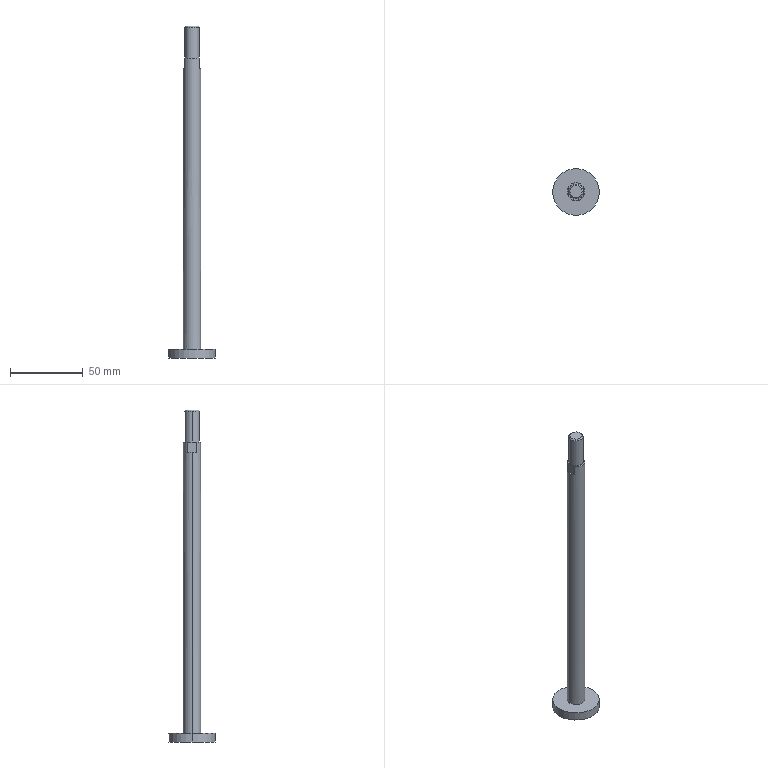Part | STEP file | 1 solid | 17 faces | box 32 x 32 x 228.2 mm | volume 29124 mm3 | plane 9 | cylinder 6 | cone 2 | commonest cylinder face diameters 10 x2 12 x2 32 x2
STEP:
#1=CARTESIAN_POINT('',(0.,0.,0.));
#2=DIRECTION('',(0.,0.,1.));
#3=DIRECTION('',(1.,0.,0.));
#4=AXIS2_PLACEMENT_3D('',#1,#2,#3);
#5=CARTESIAN_POINT('',(5.,0.,26.));
#6=VERTEX_POINT('',#5);
#7=CARTESIAN_POINT('',(-5.,0.,26.));
#8=VERTEX_POINT('',#7);
#9=CARTESIAN_POINT('',(0.,0.,26.));
#10=DIRECTION('',(0.,0.,1.));
#11=DIRECTION('',(1.,0.,0.));
#12=AXIS2_PLACEMENT_3D('',#9,#10,#11);
#13=CIRCLE('',#12,5.);
#14=CARTESIAN_POINT('',(0.,0.,26.));
#15=DIRECTION('',(0.,0.,1.));
#16=DIRECTION('',(1.,0.,0.));
#17=AXIS2_PLACEMENT_3D('',#14,#15,#16);
#18=CYLINDRICAL_SURFACE('',#17,5.);
#19=CARTESIAN_POINT('',(0.,0.));
#20=DIRECTION('',(1.,0.));
#21=VECTOR('',#20,1.);
#22=LINE('',#19,#21);
#23=(GEOMETRIC_REPRESENTATION_CONTEXT(2)PARAMETRIC_REPRESENTATION_CONTEXT()REPRESENTATION_CONTEXT('',''));
#24=DEFINITIONAL_REPRESENTATION('',(#22),#23);
#25=PCURVE('',#18,#24);
#26=CARTESIAN_POINT('',(0.,0.,26.));
#27=DIRECTION('',(0.,0.,-1.));
#28=DIRECTION('',(-1.,0.,0.));
#29=AXIS2_PLACEMENT_3D('',#26,#27,#28);
#30=PLANE('',#29);
#31=CARTESIAN_POINT('',(-5.,0.));
#32=CARTESIAN_POINT('',(-5.,8.66));
#33=CARTESIAN_POINT('',(2.5,4.33));
#34=CARTESIAN_POINT('',(10.,0.));
#35=CARTESIAN_POINT('',(2.5,-4.33));
#36=CARTESIAN_POINT('',(-5.,-8.66));
#37=CARTESIAN_POINT('',(-5.,0.));
#38=(BOUNDED_CURVE()B_SPLINE_CURVE(2,(#31,#32,#33,#34,#35,#36,#37),.UNSPECIFIED.,.T.,.F.)B_SPLINE_CURVE_WITH_KNOTS((1,2,2,2,2,1),(-2.094,0.,2.094,4.189,6.283,8.378),.UNSPECIFIED.)CURVE()GEOMETRIC_REPRESENTATION_ITEM()RATIONAL_B_SPLINE_CURVE((1.,0.5,1.,0.5,1.,0.5,1.))REPRESENTATION_ITEM(''));
#39=(GEOMETRIC_REPRESENTATION_CONTEXT(2)PARAMETRIC_REPRESENTATION_CONTEXT()REPRESENTATION_CONTEXT('',''));
#40=DEFINITIONAL_REPRESENTATION('',(#38),#39);
#41=PCURVE('',#30,#40);
#42=SURFACE_CURVE('',#13,(#25,#41),.PCURVE_S1.);
#43=EDGE_CURVE('',#6,#8,#42,.T.);
#44=ORIENTED_EDGE('',*,*,#43,.T.);
#45=CARTESIAN_POINT('',(-5.,0.,47.233));
#46=VERTEX_POINT('',#45);
#47=CARTESIAN_POINT('',(-5.,0.,26.));
#48=DIRECTION('',(0.,0.,1.));
#49=VECTOR('',#48,1.);
#50=LINE('',#47,#49);
#51=CARTESIAN_POINT('',(3.142,0.));
#52=DIRECTION('',(0.,1.));
#53=VECTOR('',#52,1.);
#54=LINE('',#51,#53);
#55=(GEOMETRIC_REPRESENTATION_CONTEXT(2)PARAMETRIC_REPRESENTATION_CONTEXT()REPRESENTATION_CONTEXT('',''));
#56=DEFINITIONAL_REPRESENTATION('',(#54),#55);
#57=PCURVE('',#18,#56);
#58=CARTESIAN_POINT('',(0.,0.,26.));
#59=DIRECTION('',(0.,0.,1.));
#60=DIRECTION('',(1.,0.,0.));
#61=AXIS2_PLACEMENT_3D('',#58,#59,#60);
#62=CYLINDRICAL_SURFACE('',#61,5.);
#63=CARTESIAN_POINT('',(3.142,0.));
#64=DIRECTION('',(0.,1.));
#65=VECTOR('',#64,1.);
#66=LINE('',#63,#65);
#67=(GEOMETRIC_REPRESENTATION_CONTEXT(2)PARAMETRIC_REPRESENTATION_CONTEXT()REPRESENTATION_CONTEXT('',''));
#68=DEFINITIONAL_REPRESENTATION('',(#66),#67);
#69=PCURVE('',#62,#68);
#70=SURFACE_CURVE('',#50,(#57,#69),.PCURVE_S1.);
#71=EDGE_CURVE('',#8,#46,#70,.T.);
#72=ORIENTED_EDGE('',*,*,#71,.T.);
#73=CARTESIAN_POINT('',(5.,0.,47.233));
#74=VERTEX_POINT('',#73);
#75=CARTESIAN_POINT('',(0.,0.,47.233));
#76=DIRECTION('',(0.,0.,1.));
#77=DIRECTION('',(1.,0.,0.));
#78=AXIS2_PLACEMENT_3D('',#75,#76,#77);
#79=CIRCLE('',#78,5.);
#80=CARTESIAN_POINT('',(0.,21.233));
#81=DIRECTION('',(1.,0.));
#82=VECTOR('',#81,1.);
#83=LINE('',#80,#82);
#84=(GEOMETRIC_REPRESENTATION_CONTEXT(2)PARAMETRIC_REPRESENTATION_CONTEXT()REPRESENTATION_CONTEXT('',''));
#85=DEFINITIONAL_REPRESENTATION('',(#83),#84);
#86=PCURVE('',#18,#85);
#87=CARTESIAN_POINT('',(0.,0.,47.233));
#88=DIRECTION('',(0.,0.,-1.));
#89=DIRECTION('',(-1.,0.,0.));
#90=AXIS2_PLACEMENT_3D('',#87,#88,#89);
#91=CONICAL_SURFACE('',#90,5.,0.7854);
#92=CARTESIAN_POINT('',(3.142,0.));
#93=DIRECTION('',(-1.,0.));
#94=VECTOR('',#93,1.);
#95=LINE('',#92,#94);
#96=(GEOMETRIC_REPRESENTATION_CONTEXT(2)PARAMETRIC_REPRESENTATION_CONTEXT()REPRESENTATION_CONTEXT('',''));
#97=DEFINITIONAL_REPRESENTATION('',(#95),#96);
#98=PCURVE('',#91,#97);
#99=SURFACE_CURVE('',#79,(#86,#98),.PCURVE_S1.);
#100=EDGE_CURVE('',#74,#46,#99,.T.);
#101=ORIENTED_EDGE('',*,*,#100,.F.);
#102=CARTESIAN_POINT('',(5.,0.,26.));
#103=DIRECTION('',(0.,0.,1.));
#104=VECTOR('',#103,1.);
#105=LINE('',#102,#104);
#106=CARTESIAN_POINT('',(0.,0.));
#107=DIRECTION('',(0.,1.));
#108=VECTOR('',#107,1.);
#109=LINE('',#106,#108);
#110=(GEOMETRIC_REPRESENTATION_CONTEXT(2)PARAMETRIC_REPRESENTATION_CONTEXT()REPRESENTATION_CONTEXT('',''));
#111=DEFINITIONAL_REPRESENTATION('',(#109),#110);
#112=PCURVE('',#18,#111);
#113=CARTESIAN_POINT('',(6.283,0.));
#114=DIRECTION('',(0.,1.));
#115=VECTOR('',#114,1.);
#116=LINE('',#113,#115);
#117=(GEOMETRIC_REPRESENTATION_CONTEXT(2)PARAMETRIC_REPRESENTATION_CONTEXT()REPRESENTATION_CONTEXT('',''));
#118=DEFINITIONAL_REPRESENTATION('',(#116),#117);
#119=PCURVE('',#62,#118);
#120=SURFACE_CURVE('',#105,(#112,#119),.PCURVE_S1.);
#121=EDGE_CURVE('',#6,#74,#120,.T.);
#122=ORIENTED_EDGE('',*,*,#121,.F.);
#123=EDGE_LOOP('',(#44,#72,#101,#122));
#124=FACE_BOUND('',#123,.T.);
#125=ADVANCED_FACE('',(#124),#18,.T.);
#126=CARTESIAN_POINT('',(4.233,0.,48.));
#127=VERTEX_POINT('',#126);
#128=CARTESIAN_POINT('',(-4.233,0.,48.));
#129=VERTEX_POINT('',#128);
#130=CARTESIAN_POINT('',(0.,0.,48.));
#131=DIRECTION('',(0.,0.,1.));
#132=DIRECTION('',(1.,0.,0.));
#133=AXIS2_PLACEMENT_3D('',#130,#131,#132);
#134=CIRCLE('',#133,4.233);
#135=CARTESIAN_POINT('',(3.142,-0.767));
#136=DIRECTION('',(-1.,0.));
#137=VECTOR('',#136,1.);
#138=LINE('',#135,#137);
#139=(GEOMETRIC_REPRESENTATION_CONTEXT(2)PARAMETRIC_REPRESENTATION_CONTEXT()REPRESENTATION_CONTEXT('',''));
#140=DEFINITIONAL_REPRESENTATION('',(#138),#139);
#141=PCURVE('',#91,#140);
#142=CARTESIAN_POINT('',(0.,0.,48.));
#143=DIRECTION('',(0.,0.,-1.));
#144=DIRECTION('',(-1.,0.,0.));
#145=AXIS2_PLACEMENT_3D('',#142,#143,#144);
#146=PLANE('',#145);
#147=CARTESIAN_POINT('',(-4.233,0.));
#148=CARTESIAN_POINT('',(-4.233,7.332));
#149=CARTESIAN_POINT('',(2.116,3.666));
#150=CARTESIAN_POINT('',(8.466,0.));
#151=CARTESIAN_POINT('',(2.116,-3.666));
#152=CARTESIAN_POINT('',(-4.233,-7.332));
#153=CARTESIAN_POINT('',(-4.233,0.));
#154=(BOUNDED_CURVE()B_SPLINE_CURVE(2,(#147,#148,#149,#150,#151,#152,#153),.UNSPECIFIED.,.T.,.F.)B_SPLINE_CURVE_WITH_KNOTS((1,2,2,2,2,1),(-2.094,0.,2.094,4.189,6.283,8.378),.UNSPECIFIED.)CURVE()GEOMETRIC_REPRESENTATION_ITEM()RATIONAL_B_SPLINE_CURVE((1.,0.5,1.,0.5,1.,0.5,1.))REPRESENTATION_ITEM(''));
#155=(GEOMETRIC_REPRESENTATION_CONTEXT(2)PARAMETRIC_REPRESENTATION_CONTEXT()REPRESENTATION_CONTEXT('',''));
#156=DEFINITIONAL_REPRESENTATION('',(#154),#155);
#157=PCURVE('',#146,#156);
#158=SURFACE_CURVE('',#134,(#141,#157),.PCURVE_S1.);
#159=EDGE_CURVE('',#127,#129,#158,.T.);
#160=ORIENTED_EDGE('',*,*,#159,.F.);
#161=CARTESIAN_POINT('',(5.,0.,47.233));
#162=DIRECTION('',(0.7071,0.,-0.7071));
#163=VECTOR('',#162,1.);
#164=LINE('',#161,#163);
#165=CARTESIAN_POINT('',(3.142,0.));
#166=DIRECTION('',(0.,1.));
#167=VECTOR('',#166,1.);
#168=LINE('',#165,#167);
#169=(GEOMETRIC_REPRESENTATION_CONTEXT(2)PARAMETRIC_REPRESENTATION_CONTEXT()REPRESENTATION_CONTEXT('',''));
#170=DEFINITIONAL_REPRESENTATION('',(#168),#169);
#171=PCURVE('',#91,#170);
#172=CARTESIAN_POINT('',(0.,0.,47.233));
#173=DIRECTION('',(0.,0.,-1.));
#174=DIRECTION('',(-1.,0.,0.));
#175=AXIS2_PLACEMENT_3D('',#172,#173,#174);
#176=CONICAL_SURFACE('',#175,5.,0.7854);
#177=CARTESIAN_POINT('',(3.142,0.));
#178=DIRECTION('',(0.,1.));
#179=VECTOR('',#178,1.);
#180=LINE('',#177,#179);
#181=(GEOMETRIC_REPRESENTATION_CONTEXT(2)PARAMETRIC_REPRESENTATION_CONTEXT()REPRESENTATION_CONTEXT('',''));
#182=DEFINITIONAL_REPRESENTATION('',(#180),#181);
#183=PCURVE('',#176,#182);
#184=SURFACE_CURVE('',#164,(#171,#183),.PCURVE_S1.);
#185=EDGE_CURVE('',#127,#74,#184,.T.);
#186=ORIENTED_EDGE('',*,*,#185,.T.);
#187=ORIENTED_EDGE('',*,*,#100,.T.);
#188=CARTESIAN_POINT('',(-5.,0.,47.233));
#189=DIRECTION('',(-0.7071,0.,-0.7071));
#190=VECTOR('',#189,1.);
#191=LINE('',#188,#190);
#192=CARTESIAN_POINT('',(0.,0.));
#193=DIRECTION('',(0.,1.));
#194=VECTOR('',#193,1.);
#195=LINE('',#192,#194);
#196=(GEOMETRIC_REPRESENTATION_CONTEXT(2)PARAMETRIC_REPRESENTATION_CONTEXT()REPRESENTATION_CONTEXT('',''));
#197=DEFINITIONAL_REPRESENTATION('',(#195),#196);
#198=PCURVE('',#91,#197);
#199=CARTESIAN_POINT('',(6.283,0.));
#200=DIRECTION('',(0.,1.));
#201=VECTOR('',#200,1.);
#202=LINE('',#199,#201);
#203=(GEOMETRIC_REPRESENTATION_CONTEXT(2)PARAMETRIC_REPRESENTATION_CONTEXT()REPRESENTATION_CONTEXT('',''));
#204=DEFINITIONAL_REPRESENTATION('',(#202),#203);
#205=PCURVE('',#176,#204);
#206=SURFACE_CURVE('',#191,(#198,#205),.PCURVE_S1.);
#207=EDGE_CURVE('',#129,#46,#206,.T.);
#208=ORIENTED_EDGE('',*,*,#207,.F.);
#209=EDGE_LOOP('',(#160,#186,#187,#208));
#210=FACE_BOUND('',#209,.T.);
#211=ADVANCED_FACE('',(#210),#91,.T.);
#212=CARTESIAN_POINT('',(16.,0.,-180.2));
#213=VERTEX_POINT('',#212);
#214=CARTESIAN_POINT('',(-16.,0.,-180.2));
#215=VERTEX_POINT('',#214);
#216=CARTESIAN_POINT('',(0.,0.,-180.2));
#217=DIRECTION('',(0.,0.,1.));
#218=DIRECTION('',(1.,0.,0.));
#219=AXIS2_PLACEMENT_3D('',#216,#217,#218);
#220=CIRCLE('',#219,16.);
#221=CARTESIAN_POINT('',(0.,0.,-180.2));
#222=DIRECTION('',(0.,0.,1.));
#223=DIRECTION('',(1.,0.,0.));
#224=AXIS2_PLACEMENT_3D('',#221,#222,#223);
#225=CYLINDRICAL_SURFACE('',#224,16.);
#226=CARTESIAN_POINT('',(0.,0.));
#227=DIRECTION('',(1.,0.));
#228=VECTOR('',#227,1.);
#229=LINE('',#226,#228);
#230=(GEOMETRIC_REPRESENTATION_CONTEXT(2)PARAMETRIC_REPRESENTATION_CONTEXT()REPRESENTATION_CONTEXT('',''));
#231=DEFINITIONAL_REPRESENTATION('',(#229),#230);
#232=PCURVE('',#225,#231);
#233=CARTESIAN_POINT('',(0.,16.,-180.2));
#234=DIRECTION('',(0.,0.,1.));
#235=DIRECTION('',(1.,0.,0.));
#236=AXIS2_PLACEMENT_3D('',#233,#234,#235);
#237=PLANE('',#236);
#238=CARTESIAN_POINT('',(0.,-16.));
#239=DIRECTION('',(1.,0.));
#240=AXIS2_PLACEMENT_2D('',#238,#239);
#241=CIRCLE('',#240,16.);
#242=(GEOMETRIC_REPRESENTATION_CONTEXT(2)PARAMETRIC_REPRESENTATION_CONTEXT()REPRESENTATION_CONTEXT('',''));
#243=DEFINITIONAL_REPRESENTATION('',(#241),#242);
#244=PCURVE('',#237,#243);
#245=SURFACE_CURVE('',#220,(#232,#244),.PCURVE_S1.);
#246=EDGE_CURVE('',#213,#215,#245,.T.);
#247=ORIENTED_EDGE('',*,*,#246,.T.);
#248=CARTESIAN_POINT('',(-16.,0.,-174.2));
#249=VERTEX_POINT('',#248);
#250=CARTESIAN_POINT('',(-16.,0.,-180.2));
#251=DIRECTION('',(0.,0.,1.));
#252=VECTOR('',#251,1.);
#253=LINE('',#250,#252);
#254=CARTESIAN_POINT('',(3.142,0.));
#255=DIRECTION('',(0.,1.));
#256=VECTOR('',#255,1.);
#257=LINE('',#254,#256);
#258=(GEOMETRIC_REPRESENTATION_CONTEXT(2)PARAMETRIC_REPRESENTATION_CONTEXT()REPRESENTATION_CONTEXT('',''));
#259=DEFINITIONAL_REPRESENTATION('',(#257),#258);
#260=PCURVE('',#225,#259);
#261=CARTESIAN_POINT('',(0.,0.,-180.2));
#262=DIRECTION('',(0.,0.,1.));
#263=DIRECTION('',(1.,0.,0.));
#264=AXIS2_PLACEMENT_3D('',#261,#262,#263);
#265=CYLINDRICAL_SURFACE('',#264,16.);
#266=CARTESIAN_POINT('',(3.142,0.));
#267=DIRECTION('',(0.,1.));
#268=VECTOR('',#267,1.);
#269=LINE('',#266,#268);
#270=(GEOMETRIC_REPRESENTATION_CONTEXT(2)PARAMETRIC_REPRESENTATION_CONTEXT()REPRESENTATION_CONTEXT('',''));
#271=DEFINITIONAL_REPRESENTATION('',(#269),#270);
#272=PCURVE('',#265,#271);
#273=SURFACE_CURVE('',#253,(#260,#272),.PCURVE_S1.);
#274=EDGE_CURVE('',#215,#249,#273,.T.);
#275=ORIENTED_EDGE('',*,*,#274,.T.);
#276=CARTESIAN_POINT('',(16.,0.,-174.2));
#277=VERTEX_POINT('',#276);
#278=CARTESIAN_POINT('',(0.,0.,-174.2));
#279=DIRECTION('',(0.,0.,1.));
#280=DIRECTION('',(1.,0.,0.));
#281=AXIS2_PLACEMENT_3D('',#278,#279,#280);
#282=CIRCLE('',#281,16.);
#283=CARTESIAN_POINT('',(0.,6.));
#284=DIRECTION('',(1.,0.));
#285=VECTOR('',#284,1.);
#286=LINE('',#283,#285);
#287=(GEOMETRIC_REPRESENTATION_CONTEXT(2)PARAMETRIC_REPRESENTATION_CONTEXT()REPRESENTATION_CONTEXT('',''));
#288=DEFINITIONAL_REPRESENTATION('',(#286),#287);
#289=PCURVE('',#225,#288);
#290=CARTESIAN_POINT('',(0.,6.,-174.2));
#291=DIRECTION('',(0.,0.,-1.));
#292=DIRECTION('',(-1.,0.,0.));
#293=AXIS2_PLACEMENT_3D('',#290,#291,#292);
#294=PLANE('',#293);
#295=CARTESIAN_POINT('',(-16.,-6.));
#296=CARTESIAN_POINT('',(-16.,21.713));
#297=CARTESIAN_POINT('',(8.,7.856));
#298=CARTESIAN_POINT('',(32.,-6.));
#299=CARTESIAN_POINT('',(8.,-19.856));
#300=CARTESIAN_POINT('',(-16.,-33.713));
#301=CARTESIAN_POINT('',(-16.,-6.));
#302=(BOUNDED_CURVE()B_SPLINE_CURVE(2,(#295,#296,#297,#298,#299,#300,#301),.UNSPECIFIED.,.T.,.F.)B_SPLINE_CURVE_WITH_KNOTS((1,2,2,2,2,1),(-2.094,0.,2.094,4.189,6.283,8.378),.UNSPECIFIED.)CURVE()GEOMETRIC_REPRESENTATION_ITEM()RATIONAL_B_SPLINE_CURVE((1.,0.5,1.,0.5,1.,0.5,1.))REPRESENTATION_ITEM(''));
#303=(GEOMETRIC_REPRESENTATION_CONTEXT(2)PARAMETRIC_REPRESENTATION_CONTEXT()REPRESENTATION_CONTEXT('',''));
#304=DEFINITIONAL_REPRESENTATION('',(#302),#303);
#305=PCURVE('',#294,#304);
#306=SURFACE_CURVE('',#282,(#289,#305),.PCURVE_S1.);
#307=EDGE_CURVE('',#277,#249,#306,.T.);
#308=ORIENTED_EDGE('',*,*,#307,.F.);
#309=CARTESIAN_POINT('',(16.,0.,-180.2));
#310=DIRECTION('',(0.,0.,1.));
#311=VECTOR('',#310,1.);
#312=LINE('',#309,#311);
#313=CARTESIAN_POINT('',(0.,0.));
#314=DIRECTION('',(0.,1.));
#315=VECTOR('',#314,1.);
#316=LINE('',#313,#315);
#317=(GEOMETRIC_REPRESENTATION_CONTEXT(2)PARAMETRIC_REPRESENTATION_CONTEXT()REPRESENTATION_CONTEXT('',''));
#318=DEFINITIONAL_REPRESENTATION('',(#316),#317);
#319=PCURVE('',#225,#318);
#320=CARTESIAN_POINT('',(6.283,0.));
#321=DIRECTION('',(0.,1.));
#322=VECTOR('',#321,1.);
#323=LINE('',#320,#322);
#324=(GEOMETRIC_REPRESENTATION_CONTEXT(2)PARAMETRIC_REPRESENTATION_CONTEXT()REPRESENTATION_CONTEXT('',''));
#325=DEFINITIONAL_REPRESENTATION('',(#323),#324);
#326=PCURVE('',#265,#325);
#327=SURFACE_CURVE('',#312,(#319,#326),.PCURVE_S1.);
#328=EDGE_CURVE('',#213,#277,#327,.T.);
#329=ORIENTED_EDGE('',*,*,#328,.F.);
#330=EDGE_LOOP('',(#247,#275,#308,#329));
#331=FACE_BOUND('',#330,.T.);
#332=ADVANCED_FACE('',(#331),#225,.T.);
#333=CARTESIAN_POINT('',(6.,0.,-174.2));
#334=VERTEX_POINT('',#333);
#335=CARTESIAN_POINT('',(-6.,0.,-174.2));
#336=VERTEX_POINT('',#335);
#337=CARTESIAN_POINT('',(0.,0.,-174.2));
#338=DIRECTION('',(0.,0.,1.));
#339=DIRECTION('',(1.,0.,0.));
#340=AXIS2_PLACEMENT_3D('',#337,#338,#339);
#341=CIRCLE('',#340,6.);
#342=CARTESIAN_POINT('',(0.,0.,-180.2));
#343=DIRECTION('',(0.,0.,1.));
#344=DIRECTION('',(1.,0.,0.));
#345=AXIS2_PLACEMENT_3D('',#342,#343,#344);
#346=CYLINDRICAL_SURFACE('',#345,6.);
#347=CARTESIAN_POINT('',(0.,6.));
#348=DIRECTION('',(1.,0.));
#349=VECTOR('',#348,1.);
#350=LINE('',#347,#349);
#351=(GEOMETRIC_REPRESENTATION_CONTEXT(2)PARAMETRIC_REPRESENTATION_CONTEXT()REPRESENTATION_CONTEXT('',''));
#352=DEFINITIONAL_REPRESENTATION('',(#350),#351);
#353=PCURVE('',#346,#352);
#354=CARTESIAN_POINT('',(-6.,-6.));
#355=CARTESIAN_POINT('',(-6.,4.392));
#356=CARTESIAN_POINT('',(3.,-0.8038));
#357=CARTESIAN_POINT('',(12.,-6.));
#358=CARTESIAN_POINT('',(3.,-11.196));
#359=CARTESIAN_POINT('',(-6.,-16.392));
#360=CARTESIAN_POINT('',(-6.,-6.));
#361=(BOUNDED_CURVE()B_SPLINE_CURVE(2,(#354,#355,#356,#357,#358,#359,#360),.UNSPECIFIED.,.T.,.F.)B_SPLINE_CURVE_WITH_KNOTS((1,2,2,2,2,1),(-2.094,0.,2.094,4.189,6.283,8.378),.UNSPECIFIED.)CURVE()GEOMETRIC_REPRESENTATION_ITEM()RATIONAL_B_SPLINE_CURVE((1.,0.5,1.,0.5,1.,0.5,1.))REPRESENTATION_ITEM(''));
#362=(GEOMETRIC_REPRESENTATION_CONTEXT(2)PARAMETRIC_REPRESENTATION_CONTEXT()REPRESENTATION_CONTEXT('',''));
#363=DEFINITIONAL_REPRESENTATION('',(#361),#362);
#364=PCURVE('',#294,#363);
#365=SURFACE_CURVE('',#341,(#353,#364),.PCURVE_S1.);
#366=EDGE_CURVE('',#334,#336,#365,.T.);
#367=ORIENTED_EDGE('',*,*,#366,.T.);
#368=CARTESIAN_POINT('',(-6.,0.,19.));
#369=VERTEX_POINT('',#368);
#370=CARTESIAN_POINT('',(-6.,0.,-180.2));
#371=DIRECTION('',(0.,0.,1.));
#372=VECTOR('',#371,1.);
#373=LINE('',#370,#372);
#374=CARTESIAN_POINT('',(3.142,0.));
#375=DIRECTION('',(0.,1.));
#376=VECTOR('',#375,1.);
#377=LINE('',#374,#376);
#378=(GEOMETRIC_REPRESENTATION_CONTEXT(2)PARAMETRIC_REPRESENTATION_CONTEXT()REPRESENTATION_CONTEXT('',''));
#379=DEFINITIONAL_REPRESENTATION('',(#377),#378);
#380=PCURVE('',#346,#379);
#381=CARTESIAN_POINT('',(0.,0.,-180.2));
#382=DIRECTION('',(0.,0.,1.));
#383=DIRECTION('',(1.,0.,0.));
#384=AXIS2_PLACEMENT_3D('',#381,#382,#383);
#385=CYLINDRICAL_SURFACE('',#384,6.);
#386=CARTESIAN_POINT('',(3.142,0.));
#387=DIRECTION('',(0.,1.));
#388=VECTOR('',#387,1.);
#389=LINE('',#386,#388);
#390=(GEOMETRIC_REPRESENTATION_CONTEXT(2)PARAMETRIC_REPRESENTATION_CONTEXT()REPRESENTATION_CONTEXT('',''));
#391=DEFINITIONAL_REPRESENTATION('',(#389),#390);
#392=PCURVE('',#385,#391);
#393=SURFACE_CURVE('',#373,(#380,#392),.PCURVE_S1.);
#394=EDGE_CURVE('',#336,#369,#393,.T.);
#395=ORIENTED_EDGE('',*,*,#394,.T.);
#396=CARTESIAN_POINT('',(-5.,3.317,19.));
#397=VERTEX_POINT('',#396);
#398=CARTESIAN_POINT('',(0.,0.,19.));
#399=DIRECTION('',(0.,0.,1.));
#400=DIRECTION('',(1.,0.,0.));
#401=AXIS2_PLACEMENT_3D('',#398,#399,#400);
#402=CIRCLE('',#401,6.);
#403=CARTESIAN_POINT('',(0.,199.2));
#404=DIRECTION('',(1.,0.));
#405=VECTOR('',#404,1.);
#406=LINE('',#403,#405);
#407=(GEOMETRIC_REPRESENTATION_CONTEXT(2)PARAMETRIC_REPRESENTATION_CONTEXT()REPRESENTATION_CONTEXT('',''));
#408=DEFINITIONAL_REPRESENTATION('',(#406),#407);
#409=PCURVE('',#346,#408);
#410=CARTESIAN_POINT('',(0.,0.,19.));
#411=DIRECTION('',(0.,0.,1.));
#412=DIRECTION('',(1.,0.,0.));
#413=AXIS2_PLACEMENT_3D('',#410,#411,#412);
#414=PLANE('',#413);
#415=CARTESIAN_POINT('',(0.,0.));
#416=DIRECTION('',(1.,0.));
#417=AXIS2_PLACEMENT_2D('',#415,#416);
#418=CIRCLE('',#417,6.);
#419=(GEOMETRIC_REPRESENTATION_CONTEXT(2)PARAMETRIC_REPRESENTATION_CONTEXT()REPRESENTATION_CONTEXT('',''));
#420=DEFINITIONAL_REPRESENTATION('',(#418),#419);
#421=PCURVE('',#414,#420);
#422=SURFACE_CURVE('',#402,(#409,#421),.PCURVE_S1.);
#423=EDGE_CURVE('',#397,#369,#422,.T.);
#424=ORIENTED_EDGE('',*,*,#423,.F.);
#425=CARTESIAN_POINT('',(-5.,3.317,26.));
#426=VERTEX_POINT('',#425);
#427=CARTESIAN_POINT('',(-5.,3.317,-180.2));
#428=DIRECTION('',(0.,0.,1.));
#429=VECTOR('',#428,1.);
#430=LINE('',#427,#429);
#431=CARTESIAN_POINT('',(2.556,0.));
#432=DIRECTION('',(0.,1.));
#433=VECTOR('',#432,1.);
#434=LINE('',#431,#433);
#435=(GEOMETRIC_REPRESENTATION_CONTEXT(2)PARAMETRIC_REPRESENTATION_CONTEXT()REPRESENTATION_CONTEXT('',''));
#436=DEFINITIONAL_REPRESENTATION('',(#434),#435);
#437=PCURVE('',#346,#436);
#438=CARTESIAN_POINT('',(-5.,-10.,19.));
#439=DIRECTION('',(1.,0.,0.));
#440=DIRECTION('',(0.,0.,-1.));
#441=AXIS2_PLACEMENT_3D('',#438,#439,#440);
#442=PLANE('',#441);
#443=CARTESIAN_POINT('',(199.2,13.317));
#444=DIRECTION('',(-1.,0.));
#445=VECTOR('',#444,1.);
#446=LINE('',#443,#445);
#447=(GEOMETRIC_REPRESENTATION_CONTEXT(2)PARAMETRIC_REPRESENTATION_CONTEXT()REPRESENTATION_CONTEXT('',''));
#448=DEFINITIONAL_REPRESENTATION('',(#446),#447);
#449=PCURVE('',#442,#448);
#450=SURFACE_CURVE('',#430,(#437,#449),.PCURVE_S1.);
#451=EDGE_CURVE('',#397,#426,#450,.T.);
#452=ORIENTED_EDGE('',*,*,#451,.T.);
#453=CARTESIAN_POINT('',(5.,3.317,26.));
#454=VERTEX_POINT('',#453);
#455=CARTESIAN_POINT('',(0.,0.,26.));
#456=DIRECTION('',(0.,0.,1.));
#457=DIRECTION('',(1.,0.,0.));
#458=AXIS2_PLACEMENT_3D('',#455,#456,#457);
#459=CIRCLE('',#458,6.);
#460=CARTESIAN_POINT('',(0.,206.2));
#461=DIRECTION('',(1.,0.));
#462=VECTOR('',#461,1.);
#463=LINE('',#460,#462);
#464=(GEOMETRIC_REPRESENTATION_CONTEXT(2)PARAMETRIC_REPRESENTATION_CONTEXT()REPRESENTATION_CONTEXT('',''));
#465=DEFINITIONAL_REPRESENTATION('',(#463),#464);
#466=PCURVE('',#346,#465);
#467=CARTESIAN_POINT('',(-6.,0.));
#468=CARTESIAN_POINT('',(-6.,10.392));
#469=CARTESIAN_POINT('',(3.,5.196));
#470=CARTESIAN_POINT('',(12.,0.));
#471=CARTESIAN_POINT('',(3.,-5.196));
#472=CARTESIAN_POINT('',(-6.,-10.392));
#473=CARTESIAN_POINT('',(-6.,0.));
#474=(BOUNDED_CURVE()B_SPLINE_CURVE(2,(#467,#468,#469,#470,#471,#472,#473),.UNSPECIFIED.,.T.,.F.)B_SPLINE_CURVE_WITH_KNOTS((1,2,2,2,2,1),(-2.094,0.,2.094,4.189,6.283,8.378),.UNSPECIFIED.)CURVE()GEOMETRIC_REPRESENTATION_ITEM()RATIONAL_B_SPLINE_CURVE((1.,0.5,1.,0.5,1.,0.5,1.))REPRESENTATION_ITEM(''));
#475=(GEOMETRIC_REPRESENTATION_CONTEXT(2)PARAMETRIC_REPRESENTATION_CONTEXT()REPRESENTATION_CONTEXT('',''));
#476=DEFINITIONAL_REPRESENTATION('',(#474),#475);
#477=PCURVE('',#30,#476);
#478=SURFACE_CURVE('',#459,(#466,#477),.PCURVE_S1.);
#479=EDGE_CURVE('',#454,#426,#478,.T.);
#480=ORIENTED_EDGE('',*,*,#479,.F.);
#481=CARTESIAN_POINT('',(5.,3.317,19.));
#482=VERTEX_POINT('',#481);
#483=CARTESIAN_POINT('',(5.,3.317,-180.2));
#484=DIRECTION('',(0.,0.,-1.));
#485=VECTOR('',#484,1.);
#486=LINE('',#483,#485);
#487=CARTESIAN_POINT('',(0.5857,0.));
#488=DIRECTION('',(0.,-1.));
#489=VECTOR('',#488,1.);
#490=LINE('',#487,#489);
#491=(GEOMETRIC_REPRESENTATION_CONTEXT(2)PARAMETRIC_REPRESENTATION_CONTEXT()REPRESENTATION_CONTEXT('',''));
#492=DEFINITIONAL_REPRESENTATION('',(#490),#491);
#493=PCURVE('',#346,#492);
#494=CARTESIAN_POINT('',(5.,10.,19.));
#495=DIRECTION('',(-1.,0.,0.));
#496=DIRECTION('',(0.,0.,1.));
#497=AXIS2_PLACEMENT_3D('',#494,#495,#496);
#498=PLANE('',#497);
#499=CARTESIAN_POINT('',(-199.2,-6.683));
#500=DIRECTION('',(-1.,0.));
#501=VECTOR('',#500,1.);
#502=LINE('',#499,#501);
#503=(GEOMETRIC_REPRESENTATION_CONTEXT(2)PARAMETRIC_REPRESENTATION_CONTEXT()REPRESENTATION_CONTEXT('',''));
#504=DEFINITIONAL_REPRESENTATION('',(#502),#503);
#505=PCURVE('',#498,#504);
#506=SURFACE_CURVE('',#486,(#493,#505),.PCURVE_S1.);
#507=EDGE_CURVE('',#454,#482,#506,.T.);
#508=ORIENTED_EDGE('',*,*,#507,.T.);
#509=CARTESIAN_POINT('',(6.,0.,19.));
#510=VERTEX_POINT('',#509);
#511=CARTESIAN_POINT('',(0.,0.,19.));
#512=DIRECTION('',(0.,0.,1.));
#513=DIRECTION('',(1.,0.,0.));
#514=AXIS2_PLACEMENT_3D('',#511,#512,#513);
#515=CIRCLE('',#514,6.);
#516=CARTESIAN_POINT('',(0.,199.2));
#517=DIRECTION('',(1.,0.));
#518=VECTOR('',#517,1.);
#519=LINE('',#516,#518);
#520=(GEOMETRIC_REPRESENTATION_CONTEXT(2)PARAMETRIC_REPRESENTATION_CONTEXT()REPRESENTATION_CONTEXT('',''));
#521=DEFINITIONAL_REPRESENTATION('',(#519),#520);
#522=PCURVE('',#346,#521);
#523=CARTESIAN_POINT('',(0.,0.,19.));
#524=DIRECTION('',(0.,0.,1.));
#525=DIRECTION('',(1.,0.,0.));
#526=AXIS2_PLACEMENT_3D('',#523,#524,#525);
#527=PLANE('',#526);
#528=CARTESIAN_POINT('',(0.,0.));
#529=DIRECTION('',(1.,0.));
#530=AXIS2_PLACEMENT_2D('',#528,#529);
#531=CIRCLE('',#530,6.);
#532=(GEOMETRIC_REPRESENTATION_CONTEXT(2)PARAMETRIC_REPRESENTATION_CONTEXT()REPRESENTATION_CONTEXT('',''));
#533=DEFINITIONAL_REPRESENTATION('',(#531),#532);
#534=PCURVE('',#527,#533);
#535=SURFACE_CURVE('',#515,(#522,#534),.PCURVE_S1.);
#536=EDGE_CURVE('',#510,#482,#535,.T.);
#537=ORIENTED_EDGE('',*,*,#536,.F.);
#538=CARTESIAN_POINT('',(6.,0.,-180.2));
#539=DIRECTION('',(0.,0.,1.));
#540=VECTOR('',#539,1.);
#541=LINE('',#538,#540);
#542=CARTESIAN_POINT('',(0.,0.));
#543=DIRECTION('',(0.,1.));
#544=VECTOR('',#543,1.);
#545=LINE('',#542,#544);
#546=(GEOMETRIC_REPRESENTATION_CONTEXT(2)PARAMETRIC_REPRESENTATION_CONTEXT()REPRESENTATION_CONTEXT('',''));
#547=DEFINITIONAL_REPRESENTATION('',(#545),#546);
#548=PCURVE('',#346,#547);
#549=CARTESIAN_POINT('',(6.283,0.));
#550=DIRECTION('',(0.,1.));
#551=VECTOR('',#550,1.);
#552=LINE('',#549,#551);
#553=(GEOMETRIC_REPRESENTATION_CONTEXT(2)PARAMETRIC_REPRESENTATION_CONTEXT()REPRESENTATION_CONTEXT('',''));
#554=DEFINITIONAL_REPRESENTATION('',(#552),#553);
#555=PCURVE('',#385,#554);
#556=SURFACE_CURVE('',#541,(#548,#555),.PCURVE_S1.);
#557=EDGE_CURVE('',#334,#510,#556,.T.);
#558=ORIENTED_EDGE('',*,*,#557,.F.);
#559=EDGE_LOOP('',(#367,#395,#424,#452,#480,#508,#537,#558));
#560=FACE_BOUND('',#559,.T.);
#561=ADVANCED_FACE('',(#560),#346,.T.);
#562=ORIENTED_EDGE('',*,*,#43,.F.);
#563=CARTESIAN_POINT('',(5.,10.,26.));
#564=DIRECTION('',(0.,-1.,0.));
#565=VECTOR('',#564,1.);
#566=LINE('',#563,#565);
#567=CARTESIAN_POINT('',(-5.,10.));
#568=DIRECTION('',(0.,-1.));
#569=VECTOR('',#568,1.);
#570=LINE('',#567,#569);
#571=(GEOMETRIC_REPRESENTATION_CONTEXT(2)PARAMETRIC_REPRESENTATION_CONTEXT()REPRESENTATION_CONTEXT('',''));
#572=DEFINITIONAL_REPRESENTATION('',(#570),#571);
#573=PCURVE('',#30,#572);
#574=CARTESIAN_POINT('',(7.,0.));
#575=DIRECTION('',(0.,-1.));
#576=VECTOR('',#575,1.);
#577=LINE('',#574,#576);
#578=(GEOMETRIC_REPRESENTATION_CONTEXT(2)PARAMETRIC_REPRESENTATION_CONTEXT()REPRESENTATION_CONTEXT('',''));
#579=DEFINITIONAL_REPRESENTATION('',(#577),#578);
#580=PCURVE('',#498,#579);
#581=SURFACE_CURVE('',#566,(#573,#580),.PCURVE_S1.);
#582=EDGE_CURVE('',#454,#6,#581,.T.);
#583=ORIENTED_EDGE('',*,*,#582,.F.);
#584=ORIENTED_EDGE('',*,*,#479,.T.);
#585=CARTESIAN_POINT('',(-5.,-10.,26.));
#586=DIRECTION('',(0.,1.,0.));
#587=VECTOR('',#586,1.);
#588=LINE('',#585,#587);
#589=CARTESIAN_POINT('',(5.,-10.));
#590=DIRECTION('',(0.,1.));
#591=VECTOR('',#590,1.);
#592=LINE('',#589,#591);
#593=(GEOMETRIC_REPRESENTATION_CONTEXT(2)PARAMETRIC_REPRESENTATION_CONTEXT()REPRESENTATION_CONTEXT('',''));
#594=DEFINITIONAL_REPRESENTATION('',(#592),#593);
#595=PCURVE('',#30,#594);
#596=CARTESIAN_POINT('',(-7.,0.));
#597=DIRECTION('',(0.,1.));
#598=VECTOR('',#597,1.);
#599=LINE('',#596,#598);
#600=(GEOMETRIC_REPRESENTATION_CONTEXT(2)PARAMETRIC_REPRESENTATION_CONTEXT()REPRESENTATION_CONTEXT('',''));
#601=DEFINITIONAL_REPRESENTATION('',(#599),#600);
#602=PCURVE('',#442,#601);
#603=SURFACE_CURVE('',#588,(#595,#602),.PCURVE_S1.);
#604=EDGE_CURVE('',#8,#426,#603,.T.);
#605=ORIENTED_EDGE('',*,*,#604,.F.);
#606=EDGE_LOOP('',(#562,#583,#584,#605));
#607=FACE_BOUND('',#606,.T.);
#608=ADVANCED_FACE('',(#607),#30,.F.);
#609=CARTESIAN_POINT('',(0.,0.,26.));
#610=DIRECTION('',(0.,0.,1.));
#611=DIRECTION('',(1.,0.,0.));
#612=AXIS2_PLACEMENT_3D('',#609,#610,#611);
#613=CIRCLE('',#612,5.);
#614=CARTESIAN_POINT('',(0.,0.,26.));
#615=DIRECTION('',(0.,0.,-1.));
#616=DIRECTION('',(-1.,0.,0.));
#617=AXIS2_PLACEMENT_3D('',#614,#615,#616);
#618=PLANE('',#617);
#619=CARTESIAN_POINT('',(-5.,0.));
#620=CARTESIAN_POINT('',(-5.,8.66));
#621=CARTESIAN_POINT('',(2.5,4.33));
#622=CARTESIAN_POINT('',(10.,0.));
#623=CARTESIAN_POINT('',(2.5,-4.33));
#624=CARTESIAN_POINT('',(-5.,-8.66));
#625=CARTESIAN_POINT('',(-5.,0.));
#626=(BOUNDED_CURVE()B_SPLINE_CURVE(2,(#619,#620,#621,#622,#623,#624,#625),.UNSPECIFIED.,.T.,.F.)B_SPLINE_CURVE_WITH_KNOTS((1,2,2,2,2,1),(-2.094,0.,2.094,4.189,6.283,8.378),.UNSPECIFIED.)CURVE()GEOMETRIC_REPRESENTATION_ITEM()RATIONAL_B_SPLINE_CURVE((1.,0.5,1.,0.5,1.,0.5,1.))REPRESENTATION_ITEM(''));
#627=(GEOMETRIC_REPRESENTATION_CONTEXT(2)PARAMETRIC_REPRESENTATION_CONTEXT()REPRESENTATION_CONTEXT('',''));
#628=DEFINITIONAL_REPRESENTATION('',(#626),#627);
#629=PCURVE('',#618,#628);
#630=CARTESIAN_POINT('',(0.,0.));
#631=DIRECTION('',(1.,0.));
#632=VECTOR('',#631,1.);
#633=LINE('',#630,#632);
#634=(GEOMETRIC_REPRESENTATION_CONTEXT(2)PARAMETRIC_REPRESENTATION_CONTEXT()REPRESENTATION_CONTEXT('',''));
#635=DEFINITIONAL_REPRESENTATION('',(#633),#634);
#636=PCURVE('',#62,#635);
#637=SURFACE_CURVE('',#613,(#629,#636),.PCURVE_S1.);
#638=EDGE_CURVE('',#8,#6,#637,.T.);
#639=ORIENTED_EDGE('',*,*,#638,.F.);
#640=CARTESIAN_POINT('',(-5.,-3.317,26.));
#641=VERTEX_POINT('',#640);
#642=CARTESIAN_POINT('',(-5.,-10.,26.));
#643=DIRECTION('',(0.,1.,0.));
#644=VECTOR('',#643,1.);
#645=LINE('',#642,#644);
#646=CARTESIAN_POINT('',(5.,-10.));
#647=DIRECTION('',(0.,1.));
#648=VECTOR('',#647,1.);
#649=LINE('',#646,#648);
#650=(GEOMETRIC_REPRESENTATION_CONTEXT(2)PARAMETRIC_REPRESENTATION_CONTEXT()REPRESENTATION_CONTEXT('',''));
#651=DEFINITIONAL_REPRESENTATION('',(#649),#650);
#652=PCURVE('',#618,#651);
#653=CARTESIAN_POINT('',(-7.,0.));
#654=DIRECTION('',(0.,1.));
#655=VECTOR('',#654,1.);
#656=LINE('',#653,#655);
#657=(GEOMETRIC_REPRESENTATION_CONTEXT(2)PARAMETRIC_REPRESENTATION_CONTEXT()REPRESENTATION_CONTEXT('',''));
#658=DEFINITIONAL_REPRESENTATION('',(#656),#657);
#659=PCURVE('',#442,#658);
#660=SURFACE_CURVE('',#645,(#652,#659),.PCURVE_S1.);
#661=EDGE_CURVE('',#641,#8,#660,.T.);
#662=ORIENTED_EDGE('',*,*,#661,.F.);
#663=CARTESIAN_POINT('',(5.,-3.317,26.));
#664=VERTEX_POINT('',#663);
#665=CARTESIAN_POINT('',(0.,0.,26.));
#666=DIRECTION('',(0.,0.,1.));
#667=DIRECTION('',(1.,0.,0.));
#668=AXIS2_PLACEMENT_3D('',#665,#666,#667);
#669=CIRCLE('',#668,6.);
#670=CARTESIAN_POINT('',(-6.,0.));
#671=CARTESIAN_POINT('',(-6.,10.392));
#672=CARTESIAN_POINT('',(3.,5.196));
#673=CARTESIAN_POINT('',(12.,0.));
#674=CARTESIAN_POINT('',(3.,-5.196));
#675=CARTESIAN_POINT('',(-6.,-10.392));
#676=CARTESIAN_POINT('',(-6.,0.));
#677=(BOUNDED_CURVE()B_SPLINE_CURVE(2,(#670,#671,#672,#673,#674,#675,#676),.UNSPECIFIED.,.T.,.F.)B_SPLINE_CURVE_WITH_KNOTS((1,2,2,2,2,1),(-2.094,0.,2.094,4.189,6.283,8.378),.UNSPECIFIED.)CURVE()GEOMETRIC_REPRESENTATION_ITEM()RATIONAL_B_SPLINE_CURVE((1.,0.5,1.,0.5,1.,0.5,1.))REPRESENTATION_ITEM(''));
#678=(GEOMETRIC_REPRESENTATION_CONTEXT(2)PARAMETRIC_REPRESENTATION_CONTEXT()REPRESENTATION_CONTEXT('',''));
#679=DEFINITIONAL_REPRESENTATION('',(#677),#678);
#680=PCURVE('',#618,#679);
#681=CARTESIAN_POINT('',(0.,206.2));
#682=DIRECTION('',(1.,0.));
#683=VECTOR('',#682,1.);
#684=LINE('',#681,#683);
#685=(GEOMETRIC_REPRESENTATION_CONTEXT(2)PARAMETRIC_REPRESENTATION_CONTEXT()REPRESENTATION_CONTEXT('',''));
#686=DEFINITIONAL_REPRESENTATION('',(#684),#685);
#687=PCURVE('',#385,#686);
#688=SURFACE_CURVE('',#669,(#680,#687),.PCURVE_S1.);
#689=EDGE_CURVE('',#641,#664,#688,.T.);
#690=ORIENTED_EDGE('',*,*,#689,.T.);
#691=CARTESIAN_POINT('',(5.,10.,26.));
#692=DIRECTION('',(0.,-1.,0.));
#693=VECTOR('',#692,1.);
#694=LINE('',#691,#693);
#695=CARTESIAN_POINT('',(-5.,10.));
#696=DIRECTION('',(0.,-1.));
#697=VECTOR('',#696,1.);
#698=LINE('',#695,#697);
#699=(GEOMETRIC_REPRESENTATION_CONTEXT(2)PARAMETRIC_REPRESENTATION_CONTEXT()REPRESENTATION_CONTEXT('',''));
#700=DEFINITIONAL_REPRESENTATION('',(#698),#699);
#701=PCURVE('',#618,#700);
#702=CARTESIAN_POINT('',(7.,0.));
#703=DIRECTION('',(0.,-1.));
#704=VECTOR('',#703,1.);
#705=LINE('',#702,#704);
#706=(GEOMETRIC_REPRESENTATION_CONTEXT(2)PARAMETRIC_REPRESENTATION_CONTEXT()REPRESENTATION_CONTEXT('',''));
#707=DEFINITIONAL_REPRESENTATION('',(#705),#706);
#708=PCURVE('',#498,#707);
#709=SURFACE_CURVE('',#694,(#701,#708),.PCURVE_S1.);
#710=EDGE_CURVE('',#6,#664,#709,.T.);
#711=ORIENTED_EDGE('',*,*,#710,.F.);
#712=EDGE_LOOP('',(#639,#662,#690,#711));
#713=FACE_BOUND('',#712,.T.);
#714=ADVANCED_FACE('',(#713),#618,.F.);
#715=ORIENTED_EDGE('',*,*,#394,.F.);
#716=CARTESIAN_POINT('',(0.,0.,-174.2));
#717=DIRECTION('',(0.,0.,1.));
#718=DIRECTION('',(1.,0.,0.));
#719=AXIS2_PLACEMENT_3D('',#716,#717,#718);
#720=CIRCLE('',#719,6.);
#721=CARTESIAN_POINT('',(0.,6.));
#722=DIRECTION('',(1.,0.));
#723=VECTOR('',#722,1.);
#724=LINE('',#721,#723);
#725=(GEOMETRIC_REPRESENTATION_CONTEXT(2)PARAMETRIC_REPRESENTATION_CONTEXT()REPRESENTATION_CONTEXT('',''));
#726=DEFINITIONAL_REPRESENTATION('',(#724),#725);
#727=PCURVE('',#385,#726);
#728=CARTESIAN_POINT('',(-6.,-6.));
#729=CARTESIAN_POINT('',(-6.,4.392));
#730=CARTESIAN_POINT('',(3.,-0.8038));
#731=CARTESIAN_POINT('',(12.,-6.));
#732=CARTESIAN_POINT('',(3.,-11.196));
#733=CARTESIAN_POINT('',(-6.,-16.392));
#734=CARTESIAN_POINT('',(-6.,-6.));
#735=(BOUNDED_CURVE()B_SPLINE_CURVE(2,(#728,#729,#730,#731,#732,#733,#734),.UNSPECIFIED.,.T.,.F.)B_SPLINE_CURVE_WITH_KNOTS((1,2,2,2,2,1),(-2.094,0.,2.094,4.189,6.283,8.378),.UNSPECIFIED.)CURVE()GEOMETRIC_REPRESENTATION_ITEM()RATIONAL_B_SPLINE_CURVE((1.,0.5,1.,0.5,1.,0.5,1.))REPRESENTATION_ITEM(''));
#736=(GEOMETRIC_REPRESENTATION_CONTEXT(2)PARAMETRIC_REPRESENTATION_CONTEXT()REPRESENTATION_CONTEXT('',''));
#737=DEFINITIONAL_REPRESENTATION('',(#735),#736);
#738=PCURVE('',#294,#737);
#739=SURFACE_CURVE('',#720,(#727,#738),.PCURVE_S1.);
#740=EDGE_CURVE('',#336,#334,#739,.T.);
#741=ORIENTED_EDGE('',*,*,#740,.T.);
#742=ORIENTED_EDGE('',*,*,#557,.T.);
#743=CARTESIAN_POINT('',(5.,-3.317,19.));
#744=VERTEX_POINT('',#743);
#745=CARTESIAN_POINT('',(0.,0.,19.));
#746=DIRECTION('',(0.,0.,1.));
#747=DIRECTION('',(1.,0.,0.));
#748=AXIS2_PLACEMENT_3D('',#745,#746,#747);
#749=CIRCLE('',#748,6.);
#750=CARTESIAN_POINT('',(0.,199.2));
#751=DIRECTION('',(1.,0.));
#752=VECTOR('',#751,1.);
#753=LINE('',#750,#752);
#754=(GEOMETRIC_REPRESENTATION_CONTEXT(2)PARAMETRIC_REPRESENTATION_CONTEXT()REPRESENTATION_CONTEXT('',''));
#755=DEFINITIONAL_REPRESENTATION('',(#753),#754);
#756=PCURVE('',#385,#755);
#757=CARTESIAN_POINT('',(0.,0.));
#758=DIRECTION('',(1.,0.));
#759=AXIS2_PLACEMENT_2D('',#757,#758);
#760=CIRCLE('',#759,6.);
#761=(GEOMETRIC_REPRESENTATION_CONTEXT(2)PARAMETRIC_REPRESENTATION_CONTEXT()REPRESENTATION_CONTEXT('',''));
#762=DEFINITIONAL_REPRESENTATION('',(#760),#761);
#763=PCURVE('',#527,#762);
#764=SURFACE_CURVE('',#749,(#756,#763),.PCURVE_S1.);
#765=EDGE_CURVE('',#744,#510,#764,.T.);
#766=ORIENTED_EDGE('',*,*,#765,.F.);
#767=CARTESIAN_POINT('',(5.,-3.317,-180.2));
#768=DIRECTION('',(0.,0.,1.));
#769=VECTOR('',#768,1.);
#770=LINE('',#767,#769);
#771=CARTESIAN_POINT('',(5.697,0.));
#772=DIRECTION('',(0.,1.));
#773=VECTOR('',#772,1.);
#774=LINE('',#771,#773);
#775=(GEOMETRIC_REPRESENTATION_CONTEXT(2)PARAMETRIC_REPRESENTATION_CONTEXT()REPRESENTATION_CONTEXT('',''));
#776=DEFINITIONAL_REPRESENTATION('',(#774),#775);
#777=PCURVE('',#385,#776);
#778=CARTESIAN_POINT('',(-199.2,-13.317));
#779=DIRECTION('',(1.,0.));
#780=VECTOR('',#779,1.);
#781=LINE('',#778,#780);
#782=(GEOMETRIC_REPRESENTATION_CONTEXT(2)PARAMETRIC_REPRESENTATION_CONTEXT()REPRESENTATION_CONTEXT('',''));
#783=DEFINITIONAL_REPRESENTATION('',(#781),#782);
#784=PCURVE('',#498,#783);
#785=SURFACE_CURVE('',#770,(#777,#784),.PCURVE_S1.);
#786=EDGE_CURVE('',#744,#664,#785,.T.);
#787=ORIENTED_EDGE('',*,*,#786,.T.);
#788=ORIENTED_EDGE('',*,*,#689,.F.);
#789=CARTESIAN_POINT('',(-5.,-3.317,19.));
#790=VERTEX_POINT('',#789);
#791=CARTESIAN_POINT('',(-5.,-3.317,-180.2));
#792=DIRECTION('',(0.,0.,-1.));
#793=VECTOR('',#792,1.);
#794=LINE('',#791,#793);
#795=CARTESIAN_POINT('',(3.727,0.));
#796=DIRECTION('',(0.,-1.));
#797=VECTOR('',#796,1.);
#798=LINE('',#795,#797);
#799=(GEOMETRIC_REPRESENTATION_CONTEXT(2)PARAMETRIC_REPRESENTATION_CONTEXT()REPRESENTATION_CONTEXT('',''));
#800=DEFINITIONAL_REPRESENTATION('',(#798),#799);
#801=PCURVE('',#385,#800);
#802=CARTESIAN_POINT('',(199.2,6.683));
#803=DIRECTION('',(1.,0.));
#804=VECTOR('',#803,1.);
#805=LINE('',#802,#804);
#806=(GEOMETRIC_REPRESENTATION_CONTEXT(2)PARAMETRIC_REPRESENTATION_CONTEXT()REPRESENTATION_CONTEXT('',''));
#807=DEFINITIONAL_REPRESENTATION('',(#805),#806);
#808=PCURVE('',#442,#807);
#809=SURFACE_CURVE('',#794,(#801,#808),.PCURVE_S1.);
#810=EDGE_CURVE('',#641,#790,#809,.T.);
#811=ORIENTED_EDGE('',*,*,#810,.T.);
#812=CARTESIAN_POINT('',(0.,0.,19.));
#813=DIRECTION('',(0.,0.,1.));
#814=DIRECTION('',(1.,0.,0.));
#815=AXIS2_PLACEMENT_3D('',#812,#813,#814);
#816=CIRCLE('',#815,6.);
#817=CARTESIAN_POINT('',(0.,199.2));
#818=DIRECTION('',(1.,0.));
#819=VECTOR('',#818,1.);
#820=LINE('',#817,#819);
#821=(GEOMETRIC_REPRESENTATION_CONTEXT(2)PARAMETRIC_REPRESENTATION_CONTEXT()REPRESENTATION_CONTEXT('',''));
#822=DEFINITIONAL_REPRESENTATION('',(#820),#821);
#823=PCURVE('',#385,#822);
#824=CARTESIAN_POINT('',(0.,0.));
#825=DIRECTION('',(1.,0.));
#826=AXIS2_PLACEMENT_2D('',#824,#825);
#827=CIRCLE('',#826,6.);
#828=(GEOMETRIC_REPRESENTATION_CONTEXT(2)PARAMETRIC_REPRESENTATION_CONTEXT()REPRESENTATION_CONTEXT('',''));
#829=DEFINITIONAL_REPRESENTATION('',(#827),#828);
#830=PCURVE('',#414,#829);
#831=SURFACE_CURVE('',#816,(#823,#830),.PCURVE_S1.);
#832=EDGE_CURVE('',#369,#790,#831,.T.);
#833=ORIENTED_EDGE('',*,*,#832,.F.);
#834=EDGE_LOOP('',(#715,#741,#742,#766,#787,#788,#811,#833));
#835=FACE_BOUND('',#834,.T.);
#836=ADVANCED_FACE('',(#835),#385,.T.);
#837=ORIENTED_EDGE('',*,*,#366,.F.);
#838=ORIENTED_EDGE('',*,*,#740,.F.);
#839=EDGE_LOOP('',(#837,#838));
#840=FACE_BOUND('',#839,.T.);
#841=ORIENTED_EDGE('',*,*,#307,.T.);
#842=CARTESIAN_POINT('',(0.,0.,-174.2));
#843=DIRECTION('',(0.,0.,1.));
#844=DIRECTION('',(1.,0.,0.));
#845=AXIS2_PLACEMENT_3D('',#842,#843,#844);
#846=CIRCLE('',#845,16.);
#847=CARTESIAN_POINT('',(-16.,-6.));
#848=CARTESIAN_POINT('',(-16.,21.713));
#849=CARTESIAN_POINT('',(8.,7.856));
#850=CARTESIAN_POINT('',(32.,-6.));
#851=CARTESIAN_POINT('',(8.,-19.856));
#852=CARTESIAN_POINT('',(-16.,-33.713));
#853=CARTESIAN_POINT('',(-16.,-6.));
#854=(BOUNDED_CURVE()B_SPLINE_CURVE(2,(#847,#848,#849,#850,#851,#852,#853),.UNSPECIFIED.,.T.,.F.)B_SPLINE_CURVE_WITH_KNOTS((1,2,2,2,2,1),(-2.094,0.,2.094,4.189,6.283,8.378),.UNSPECIFIED.)CURVE()GEOMETRIC_REPRESENTATION_ITEM()RATIONAL_B_SPLINE_CURVE((1.,0.5,1.,0.5,1.,0.5,1.))REPRESENTATION_ITEM(''));
#855=(GEOMETRIC_REPRESENTATION_CONTEXT(2)PARAMETRIC_REPRESENTATION_CONTEXT()REPRESENTATION_CONTEXT('',''));
#856=DEFINITIONAL_REPRESENTATION('',(#854),#855);
#857=PCURVE('',#294,#856);
#858=CARTESIAN_POINT('',(0.,6.));
#859=DIRECTION('',(1.,0.));
#860=VECTOR('',#859,1.);
#861=LINE('',#858,#860);
#862=(GEOMETRIC_REPRESENTATION_CONTEXT(2)PARAMETRIC_REPRESENTATION_CONTEXT()REPRESENTATION_CONTEXT('',''));
#863=DEFINITIONAL_REPRESENTATION('',(#861),#862);
#864=PCURVE('',#265,#863);
#865=SURFACE_CURVE('',#846,(#857,#864),.PCURVE_S1.);
#866=EDGE_CURVE('',#249,#277,#865,.T.);
#867=ORIENTED_EDGE('',*,*,#866,.T.);
#868=EDGE_LOOP('',(#841,#867));
#869=FACE_BOUND('',#868,.T.);
#870=ADVANCED_FACE('',(#840,#869),#294,.F.);
#871=ORIENTED_EDGE('',*,*,#274,.F.);
#872=CARTESIAN_POINT('',(0.,0.,-180.2));
#873=DIRECTION('',(0.,0.,1.));
#874=DIRECTION('',(1.,0.,0.));
#875=AXIS2_PLACEMENT_3D('',#872,#873,#874);
#876=CIRCLE('',#875,16.);
#877=CARTESIAN_POINT('',(0.,0.));
#878=DIRECTION('',(1.,0.));
#879=VECTOR('',#878,1.);
#880=LINE('',#877,#879);
#881=(GEOMETRIC_REPRESENTATION_CONTEXT(2)PARAMETRIC_REPRESENTATION_CONTEXT()REPRESENTATION_CONTEXT('',''));
#882=DEFINITIONAL_REPRESENTATION('',(#880),#881);
#883=PCURVE('',#265,#882);
#884=CARTESIAN_POINT('',(0.,-16.));
#885=DIRECTION('',(1.,0.));
#886=AXIS2_PLACEMENT_2D('',#884,#885);
#887=CIRCLE('',#886,16.);
#888=(GEOMETRIC_REPRESENTATION_CONTEXT(2)PARAMETRIC_REPRESENTATION_CONTEXT()REPRESENTATION_CONTEXT('',''));
#889=DEFINITIONAL_REPRESENTATION('',(#887),#888);
#890=PCURVE('',#237,#889);
#891=SURFACE_CURVE('',#876,(#883,#890),.PCURVE_S1.);
#892=EDGE_CURVE('',#215,#213,#891,.T.);
#893=ORIENTED_EDGE('',*,*,#892,.T.);
#894=ORIENTED_EDGE('',*,*,#328,.T.);
#895=ORIENTED_EDGE('',*,*,#866,.F.);
#896=EDGE_LOOP('',(#871,#893,#894,#895));
#897=FACE_BOUND('',#896,.T.);
#898=ADVANCED_FACE('',(#897),#265,.T.);
#899=ORIENTED_EDGE('',*,*,#246,.F.);
#900=ORIENTED_EDGE('',*,*,#892,.F.);
#901=EDGE_LOOP('',(#899,#900));
#902=FACE_BOUND('',#901,.T.);
#903=ADVANCED_FACE('',(#902),#237,.F.);
#904=ORIENTED_EDGE('',*,*,#765,.T.);
#905=ORIENTED_EDGE('',*,*,#536,.T.);
#906=CARTESIAN_POINT('',(5.,10.,19.));
#907=DIRECTION('',(0.,-1.,0.));
#908=VECTOR('',#907,1.);
#909=LINE('',#906,#908);
#910=CARTESIAN_POINT('',(5.,10.));
#911=DIRECTION('',(0.,-1.));
#912=VECTOR('',#911,1.);
#913=LINE('',#910,#912);
#914=(GEOMETRIC_REPRESENTATION_CONTEXT(2)PARAMETRIC_REPRESENTATION_CONTEXT()REPRESENTATION_CONTEXT('',''));
#915=DEFINITIONAL_REPRESENTATION('',(#913),#914);
#916=PCURVE('',#527,#915);
#917=CARTESIAN_POINT('',(0.,0.));
#918=DIRECTION('',(0.,-1.));
#919=VECTOR('',#918,1.);
#920=LINE('',#917,#919);
#921=(GEOMETRIC_REPRESENTATION_CONTEXT(2)PARAMETRIC_REPRESENTATION_CONTEXT()REPRESENTATION_CONTEXT('',''));
#922=DEFINITIONAL_REPRESENTATION('',(#920),#921);
#923=PCURVE('',#498,#922);
#924=SURFACE_CURVE('',#909,(#916,#923),.PCURVE_S1.);
#925=EDGE_CURVE('',#482,#744,#924,.T.);
#926=ORIENTED_EDGE('',*,*,#925,.T.);
#927=EDGE_LOOP('',(#904,#905,#926));
#928=FACE_BOUND('',#927,.T.);
#929=ADVANCED_FACE('',(#928),#527,.T.);
#930=ORIENTED_EDGE('',*,*,#925,.F.);
#931=ORIENTED_EDGE('',*,*,#507,.F.);
#932=ORIENTED_EDGE('',*,*,#582,.T.);
#933=ORIENTED_EDGE('',*,*,#710,.T.);
#934=ORIENTED_EDGE('',*,*,#786,.F.);
#935=EDGE_LOOP('',(#930,#931,#932,#933,#934));
#936=FACE_BOUND('',#935,.T.);
#937=ADVANCED_FACE('',(#936),#498,.F.);
#938=CARTESIAN_POINT('',(-5.,-10.,19.));
#939=DIRECTION('',(0.,1.,0.));
#940=VECTOR('',#939,1.);
#941=LINE('',#938,#940);
#942=CARTESIAN_POINT('',(0.,0.));
#943=DIRECTION('',(0.,1.));
#944=VECTOR('',#943,1.);
#945=LINE('',#942,#944);
#946=(GEOMETRIC_REPRESENTATION_CONTEXT(2)PARAMETRIC_REPRESENTATION_CONTEXT()REPRESENTATION_CONTEXT('',''));
#947=DEFINITIONAL_REPRESENTATION('',(#945),#946);
#948=PCURVE('',#442,#947);
#949=CARTESIAN_POINT('',(-5.,-10.));
#950=DIRECTION('',(0.,1.));
#951=VECTOR('',#950,1.);
#952=LINE('',#949,#951);
#953=(GEOMETRIC_REPRESENTATION_CONTEXT(2)PARAMETRIC_REPRESENTATION_CONTEXT()REPRESENTATION_CONTEXT('',''));
#954=DEFINITIONAL_REPRESENTATION('',(#952),#953);
#955=PCURVE('',#414,#954);
#956=SURFACE_CURVE('',#941,(#948,#955),.PCURVE_S1.);
#957=EDGE_CURVE('',#790,#397,#956,.T.);
#958=ORIENTED_EDGE('',*,*,#957,.F.);
#959=ORIENTED_EDGE('',*,*,#810,.F.);
#960=ORIENTED_EDGE('',*,*,#661,.T.);
#961=ORIENTED_EDGE('',*,*,#604,.T.);
#962=ORIENTED_EDGE('',*,*,#451,.F.);
#963=EDGE_LOOP('',(#958,#959,#960,#961,#962));
#964=FACE_BOUND('',#963,.T.);
#965=ADVANCED_FACE('',(#964),#442,.F.);
#966=ORIENTED_EDGE('',*,*,#423,.T.);
#967=ORIENTED_EDGE('',*,*,#832,.T.);
#968=ORIENTED_EDGE('',*,*,#957,.T.);
#969=EDGE_LOOP('',(#966,#967,#968));
#970=FACE_BOUND('',#969,.T.);
#971=ADVANCED_FACE('',(#970),#414,.T.);
#972=CARTESIAN_POINT('',(0.,0.,48.));
#973=DIRECTION('',(0.,0.,1.));
#974=DIRECTION('',(1.,0.,0.));
#975=AXIS2_PLACEMENT_3D('',#972,#973,#974);
#976=CIRCLE('',#975,4.233);
#977=CARTESIAN_POINT('',(-4.233,0.));
#978=CARTESIAN_POINT('',(-4.233,7.332));
#979=CARTESIAN_POINT('',(2.116,3.666));
#980=CARTESIAN_POINT('',(8.466,0.));
#981=CARTESIAN_POINT('',(2.116,-3.666));
#982=CARTESIAN_POINT('',(-4.233,-7.332));
#983=CARTESIAN_POINT('',(-4.233,0.));
#984=(BOUNDED_CURVE()B_SPLINE_CURVE(2,(#977,#978,#979,#980,#981,#982,#983),.UNSPECIFIED.,.T.,.F.)B_SPLINE_CURVE_WITH_KNOTS((1,2,2,2,2,1),(-2.094,0.,2.094,4.189,6.283,8.378),.UNSPECIFIED.)CURVE()GEOMETRIC_REPRESENTATION_ITEM()RATIONAL_B_SPLINE_CURVE((1.,0.5,1.,0.5,1.,0.5,1.))REPRESENTATION_ITEM(''));
#985=(GEOMETRIC_REPRESENTATION_CONTEXT(2)PARAMETRIC_REPRESENTATION_CONTEXT()REPRESENTATION_CONTEXT('',''));
#986=DEFINITIONAL_REPRESENTATION('',(#984),#985);
#987=PCURVE('',#146,#986);
#988=CARTESIAN_POINT('',(9.425,-0.767));
#989=DIRECTION('',(-1.,0.));
#990=VECTOR('',#989,1.);
#991=LINE('',#988,#990);
#992=(GEOMETRIC_REPRESENTATION_CONTEXT(2)PARAMETRIC_REPRESENTATION_CONTEXT()REPRESENTATION_CONTEXT('',''));
#993=DEFINITIONAL_REPRESENTATION('',(#991),#992);
#994=PCURVE('',#176,#993);
#995=SURFACE_CURVE('',#976,(#987,#994),.PCURVE_S1.);
#996=EDGE_CURVE('',#129,#127,#995,.T.);
#997=ORIENTED_EDGE('',*,*,#996,.T.);
#998=ORIENTED_EDGE('',*,*,#159,.T.);
#999=EDGE_LOOP('',(#997,#998));
#1000=FACE_BOUND('',#999,.T.);
#1001=ADVANCED_FACE('',(#1000),#146,.F.);
#1002=ORIENTED_EDGE('',*,*,#185,.F.);
#1003=ORIENTED_EDGE('',*,*,#996,.F.);
#1004=ORIENTED_EDGE('',*,*,#207,.T.);
#1005=CARTESIAN_POINT('',(0.,0.,47.233));
#1006=DIRECTION('',(0.,0.,1.));
#1007=DIRECTION('',(1.,0.,0.));
#1008=AXIS2_PLACEMENT_3D('',#1005,#1006,#1007);
#1009=CIRCLE('',#1008,5.);
#1010=CARTESIAN_POINT('',(9.425,0.));
#1011=DIRECTION('',(-1.,0.));
#1012=VECTOR('',#1011,1.);
#1013=LINE('',#1010,#1012);
#1014=(GEOMETRIC_REPRESENTATION_CONTEXT(2)PARAMETRIC_REPRESENTATION_CONTEXT()REPRESENTATION_CONTEXT('',''));
#1015=DEFINITIONAL_REPRESENTATION('',(#1013),#1014);
#1016=PCURVE('',#176,#1015);
#1017=CARTESIAN_POINT('',(0.,21.233));
#1018=DIRECTION('',(1.,0.));
#1019=VECTOR('',#1018,1.);
#1020=LINE('',#1017,#1019);
#1021=(GEOMETRIC_REPRESENTATION_CONTEXT(2)PARAMETRIC_REPRESENTATION_CONTEXT()REPRESENTATION_CONTEXT('',''));
#1022=DEFINITIONAL_REPRESENTATION('',(#1020),#1021);
#1023=PCURVE('',#62,#1022);
#1024=SURFACE_CURVE('',#1009,(#1016,#1023),.PCURVE_S1.);
#1025=EDGE_CURVE('',#46,#74,#1024,.T.);
#1026=ORIENTED_EDGE('',*,*,#1025,.T.);
#1027=EDGE_LOOP('',(#1002,#1003,#1004,#1026));
#1028=FACE_BOUND('',#1027,.T.);
#1029=ADVANCED_FACE('',(#1028),#176,.T.);
#1030=ORIENTED_EDGE('',*,*,#71,.F.);
#1031=ORIENTED_EDGE('',*,*,#638,.T.);
#1032=ORIENTED_EDGE('',*,*,#121,.T.);
#1033=ORIENTED_EDGE('',*,*,#1025,.F.);
#1034=EDGE_LOOP('',(#1030,#1031,#1032,#1033));
#1035=FACE_BOUND('',#1034,.T.);
#1036=ADVANCED_FACE('',(#1035),#62,.T.);
#1037=CLOSED_SHELL('',(#125,#211,#332,#561,#608,#714,#836,#870,#898,#903,#929,#937,#965,#971,#1001,#1029,#1036));
#1038=MANIFOLD_SOLID_BREP('',#1037);
#1039=(LENGTH_UNIT()NAMED_UNIT(*)SI_UNIT(.MILLI.,.METRE.));
#1040=UNCERTAINTY_MEASURE_WITH_UNIT(LENGTH_MEASURE(0.0000001),#1039,'','');
#1041=(NAMED_UNIT(*)PLANE_ANGLE_UNIT()SI_UNIT($,.RADIAN.));
#1042=(NAMED_UNIT(*)SI_UNIT($,.STERADIAN.)SOLID_ANGLE_UNIT());
#1043=(GEOMETRIC_REPRESENTATION_CONTEXT(3)GLOBAL_UNCERTAINTY_ASSIGNED_CONTEXT((#1040))GLOBAL_UNIT_ASSIGNED_CONTEXT((#1039,#1041,#1042))REPRESENTATION_CONTEXT('',''));
#1044=ADVANCED_BREP_SHAPE_REPRESENTATION('',(#4,#1038),#1043);